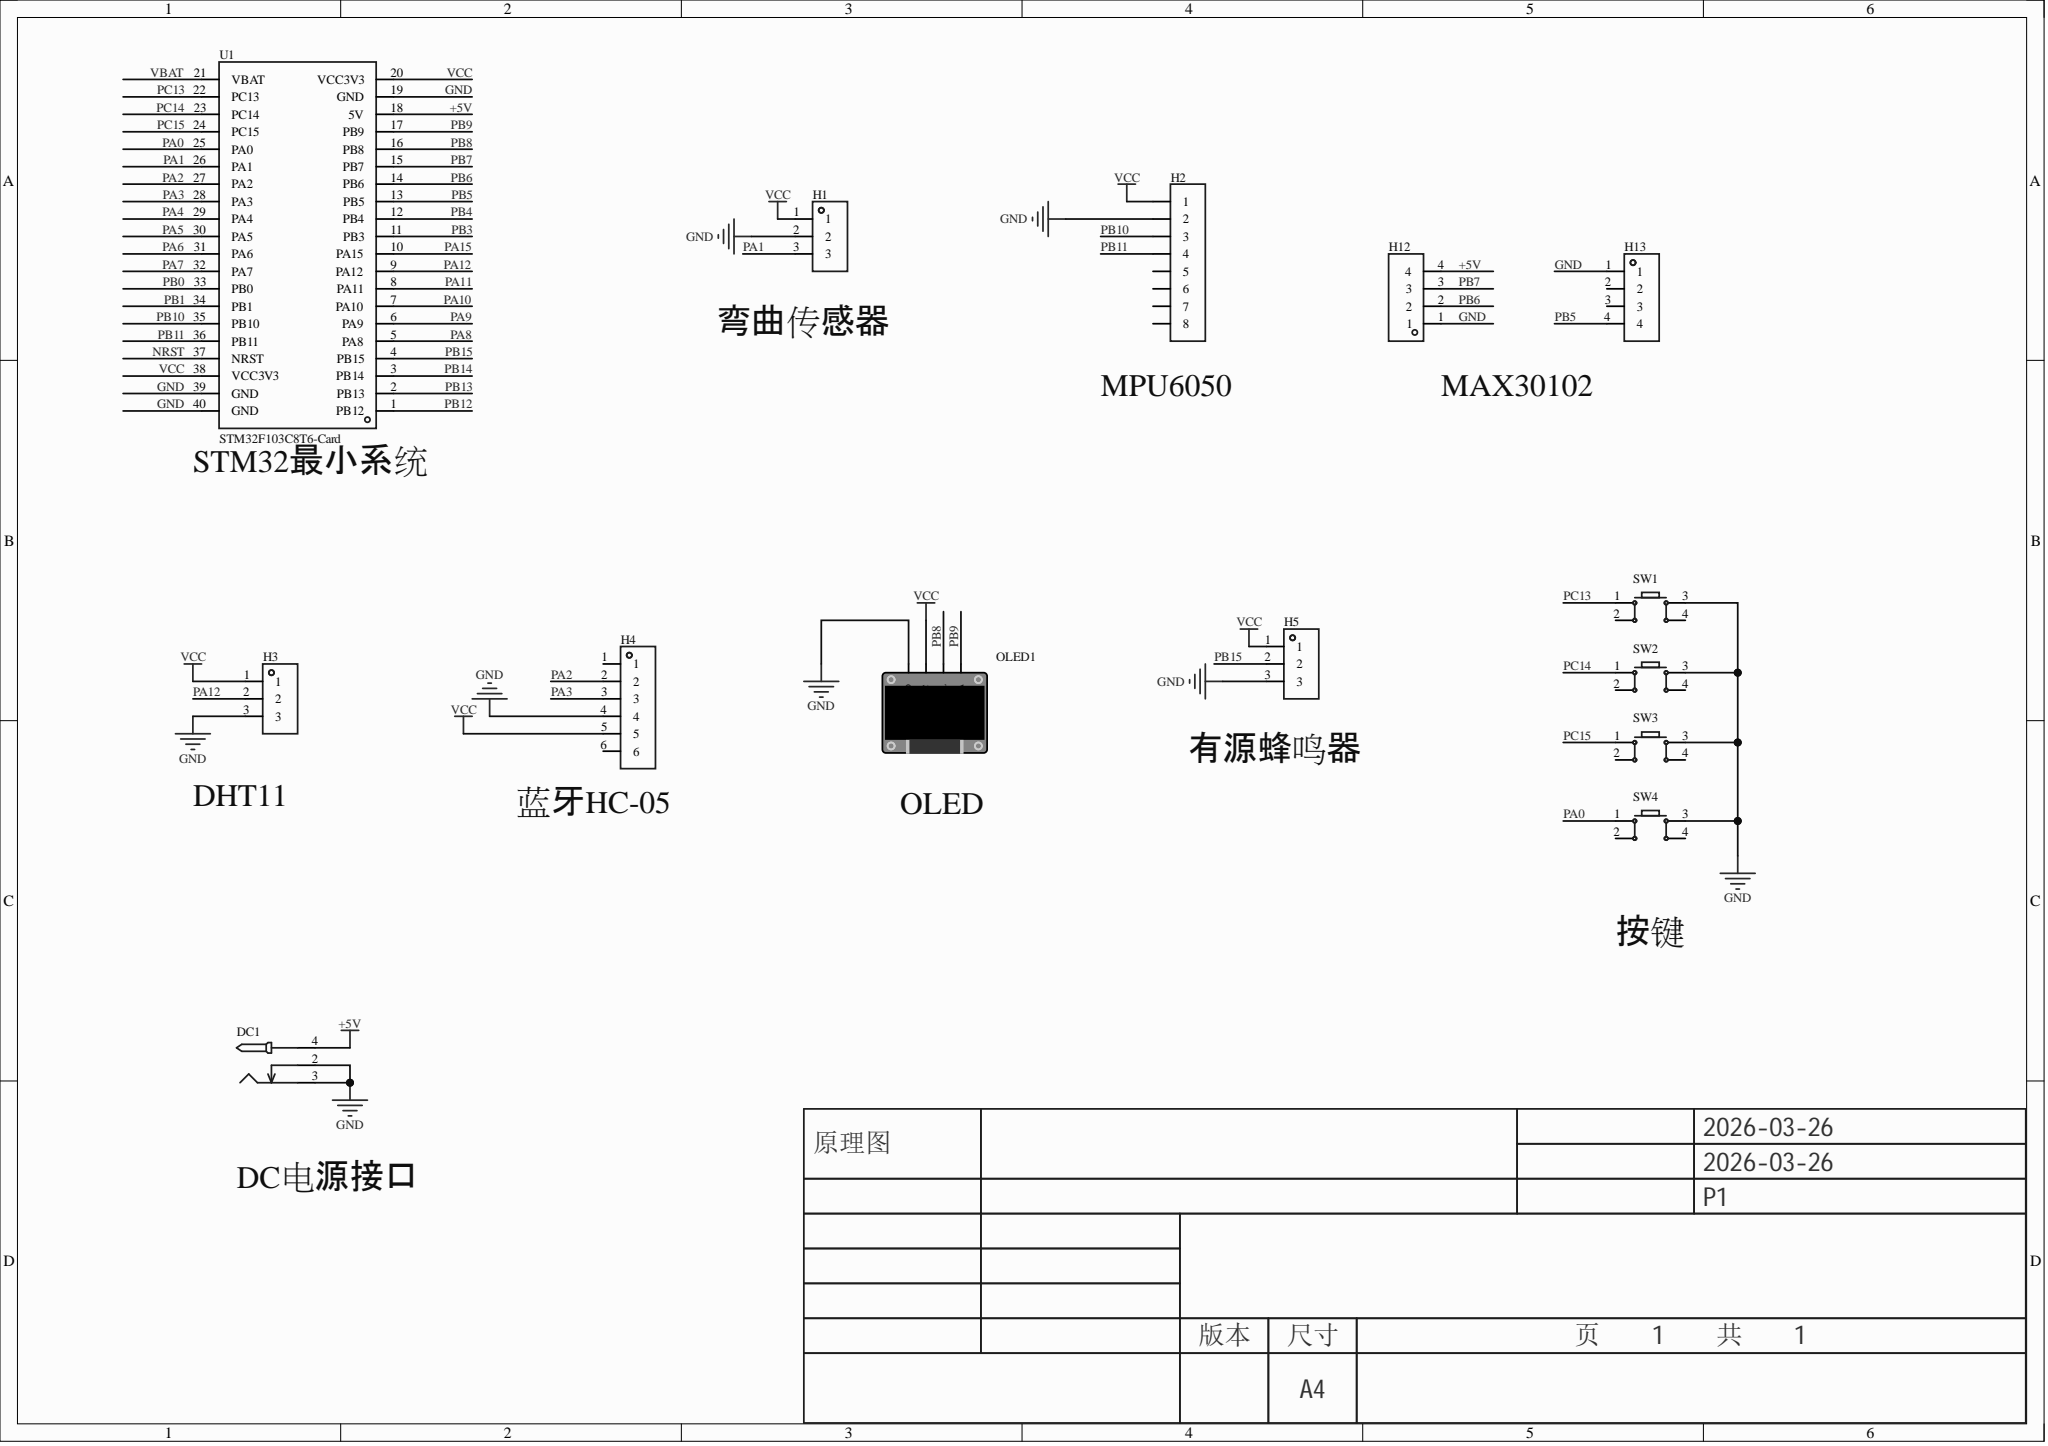Circuit board | Altium Designer | 14 parts | 19 nets
Bill of materials:
Comment,Description,Designator,Footprint,LibRef,Quantity
"","","DC1","DC-2.0","DC-005_2.0","1"
"","","H1, H3, H5","HDR-TH_3P-P2.54-V-F","HDR-F_2.54_1x3P","3"
"","","H2","HDR-TH_8P-P2.54-V-F-1","HDR-F_2.54_1x8P","1"
"","","H4","HDR-TH_6P-P2.54-V-F","HDR-F_2.54_1x6P","1"
"","","H12, H13","HDR-TH_4P-P2.54-V-F","HDR-F_2.54_1x4P","2"
"","","OLED1","0.96OLED_4P","0.96OLED模块_4P","1"
"","","SW1, SW2, SW3, SW4","SW-TH_4P-L6.0-W6.0-P4.50-LS6.5","Key_TH_6x6x6","4"
"STM32F103C8T6-Card","","U1","CONN-TH_L53.3-W22.9_STM32F103C8T6-CARD","STM32F103C8T6-Card","1"
Netlist (Protel format):
[
DC1
DC-2.0




]
[
H1
HDR-TH_3P-P2.54-V-F




]
[
H2
HDR-TH_8P-P2.54-V-F-1




]
[
H3
HDR-TH_3P-P2.54-V-F




]
[
H4
HDR-TH_6P-P2.54-V-F




]
[
H5
HDR-TH_3P-P2.54-V-F




]
[
H12
HDR-TH_4P-P2.54-V-F




]
[
H13
HDR-TH_4P-P2.54-V-F




]
[
OLED1
0.96OLED_4P




]
[
SW1
SW-TH_4P-L6.0-W6.0-P4.50-LS6.5




]
[
SW2
SW-TH_4P-L6.0-W6.0-P4.50-LS6.5




]
[
SW3
SW-TH_4P-L6.0-W6.0-P4.50-LS6.5




]
[
SW4
SW-TH_4P-L6.0-W6.0-P4.50-LS6.5




]
[
U1
CONN-TH_L53.3-W22.9_STM32F103C8T6-CARD
STM32F103C8T6-Card



]
(
VCC
H1-1
H2-1
H3-1
H4-5
H5-1
OLED1-2
U1-20
U1-38
)
(
PC15
SW3-1
U1-24
)
(
PC14
SW2-1
U1-23
)
(
PC13
SW1-1
U1-22
)
(
PB15
H5-2
U1-4
)
(
PB11
H2-4
U1-36
)
(
PB10
H2-3
U1-35
)
(
PB9
OLED1-4
U1-17
)
(
PB8
OLED1-3
U1-16
)
(
PB7
H12-3
U1-15
)
(
PB6
H12-2
U1-14
)
(
PB5
H13-4
U1-13
)
(
PA12
H3-2
U1-9
)
(
PA3
H4-3
U1-28
)
(
PA2
H4-2
U1-27
)
(
PA1
H1-3
U1-26
)
(
PA0
SW4-1
U1-25
)
(
GND
DC1-2
DC1-3
H1-2
H2-2
H3-3
H4-4
H5-3
H12-1
H13-1
OLED1-1
SW1-3
SW2-3
SW3-3
SW4-3
U1-19
U1-39
U1-40
)
(
+5V
DC1-4
H12-4
U1-18
)